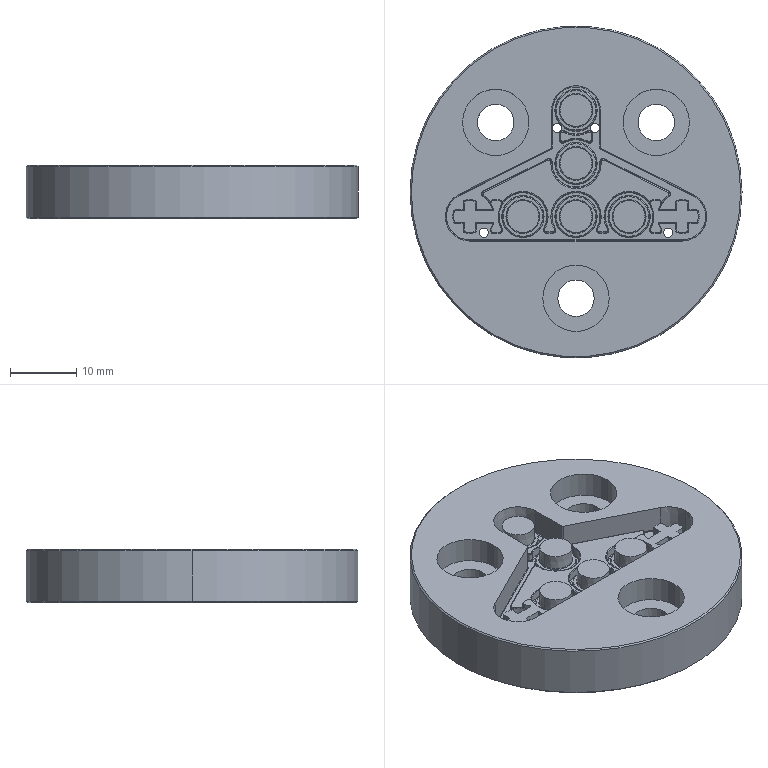Part | STEP file | Core | 1 solid | 392 faces | box 50 x 50 x 8 mm | volume 13150 mm3 | torus 124 | cone 100 | cylinder 71 | plane 59 | spline 32 | sphere 6 | commonest cylinder face diameters 0.201 x49 1.4 x8 5.5 x6 10 x6 50 x2